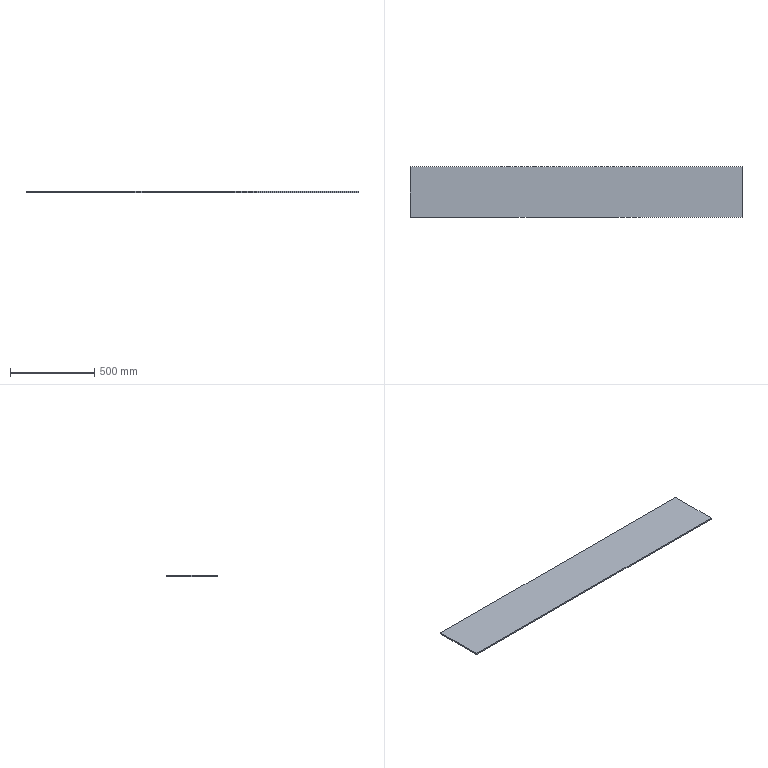Part | SolidWorks | features BaseBody 1, MoveFace 1 | 1 solid | 6 faces | box 1968 x 300 x 8 mm | volume 4723200 mm3 | plane 6
STEP:
#1=CARTESIAN_POINT('',(0.,0.,0.));
#2=VERTEX_POINT('',#1);
#3=CARTESIAN_POINT('',(1968.,0.,0.));
#4=VERTEX_POINT('',#3);
#5=CARTESIAN_POINT('',(0.,0.,0.));
#6=DIRECTION('',(1.,0.,0.));
#7=VECTOR('',#6,1000.);
#8=LINE('',#5,#7);
#9=EDGE_CURVE('',#2,#4,#8,.T.);
#10=ORIENTED_EDGE('',*,*,#9,.F.);
#11=CARTESIAN_POINT('',(0.,300.,0.));
#12=VERTEX_POINT('',#11);
#13=CARTESIAN_POINT('',(0.,300.,0.));
#14=DIRECTION('',(0.,-1.,0.));
#15=VECTOR('',#14,1000.);
#16=LINE('',#13,#15);
#17=EDGE_CURVE('',#12,#2,#16,.T.);
#18=ORIENTED_EDGE('',*,*,#17,.F.);
#19=CARTESIAN_POINT('',(1968.,300.,0.));
#20=VERTEX_POINT('',#19);
#21=CARTESIAN_POINT('',(1970.,300.,0.));
#22=DIRECTION('',(-1.,0.,0.));
#23=VECTOR('',#22,1000.);
#24=LINE('',#21,#23);
#25=EDGE_CURVE('',#20,#12,#24,.T.);
#26=ORIENTED_EDGE('',*,*,#25,.F.);
#27=CARTESIAN_POINT('',(1968.,0.,0.));
#28=DIRECTION('',(0.,1.,0.));
#29=VECTOR('',#28,1000.);
#30=LINE('',#27,#29);
#31=EDGE_CURVE('',#4,#20,#30,.T.);
#32=ORIENTED_EDGE('',*,*,#31,.F.);
#33=EDGE_LOOP('',(#10,#18,#26,#32));
#34=FACE_OUTER_BOUND('',#33,.T.);
#35=CARTESIAN_POINT('',(985.,150.,0.));
#36=DIRECTION('',(0.,0.,1.));
#37=DIRECTION('',(1.,0.,0.));
#38=AXIS2_PLACEMENT_3D('',#35,#36,#37);
#39=PLANE('',#38);
#40=ADVANCED_FACE('',(#34),#39,.F.);
#41=CARTESIAN_POINT('',(0.,0.,8.));
#42=VERTEX_POINT('',#41);
#43=CARTESIAN_POINT('',(1968.,0.,8.));
#44=VERTEX_POINT('',#43);
#45=CARTESIAN_POINT('',(0.,0.,8.));
#46=DIRECTION('',(1.,0.,0.));
#47=VECTOR('',#46,1000.);
#48=LINE('',#45,#47);
#49=EDGE_CURVE('',#42,#44,#48,.T.);
#50=ORIENTED_EDGE('',*,*,#49,.T.);
#51=CARTESIAN_POINT('',(1968.,300.,8.));
#52=VERTEX_POINT('',#51);
#53=CARTESIAN_POINT('',(1968.,0.,8.));
#54=DIRECTION('',(0.,1.,0.));
#55=VECTOR('',#54,1000.);
#56=LINE('',#53,#55);
#57=EDGE_CURVE('',#44,#52,#56,.T.);
#58=ORIENTED_EDGE('',*,*,#57,.T.);
#59=CARTESIAN_POINT('',(0.,300.,8.));
#60=VERTEX_POINT('',#59);
#61=CARTESIAN_POINT('',(1970.,300.,8.));
#62=DIRECTION('',(-1.,0.,0.));
#63=VECTOR('',#62,1000.);
#64=LINE('',#61,#63);
#65=EDGE_CURVE('',#52,#60,#64,.T.);
#66=ORIENTED_EDGE('',*,*,#65,.T.);
#67=CARTESIAN_POINT('',(0.,300.,8.));
#68=DIRECTION('',(0.,-1.,0.));
#69=VECTOR('',#68,1000.);
#70=LINE('',#67,#69);
#71=EDGE_CURVE('',#60,#42,#70,.T.);
#72=ORIENTED_EDGE('',*,*,#71,.T.);
#73=EDGE_LOOP('',(#50,#58,#66,#72));
#74=FACE_OUTER_BOUND('',#73,.T.);
#75=CARTESIAN_POINT('',(985.,150.,8.));
#76=DIRECTION('',(0.,0.,1.));
#77=DIRECTION('',(1.,0.,0.));
#78=AXIS2_PLACEMENT_3D('',#75,#76,#77);
#79=PLANE('',#78);
#80=ADVANCED_FACE('',(#74),#79,.T.);
#81=ORIENTED_EDGE('',*,*,#9,.T.);
#82=CARTESIAN_POINT('',(1968.,0.,0.));
#83=DIRECTION('',(0.,0.,1.));
#84=VECTOR('',#83,1000.);
#85=LINE('',#82,#84);
#86=EDGE_CURVE('',#4,#44,#85,.T.);
#87=ORIENTED_EDGE('',*,*,#86,.T.);
#88=ORIENTED_EDGE('',*,*,#49,.F.);
#89=CARTESIAN_POINT('',(0.,0.,0.));
#90=DIRECTION('',(0.,0.,1.));
#91=VECTOR('',#90,1000.);
#92=LINE('',#89,#91);
#93=EDGE_CURVE('',#2,#42,#92,.T.);
#94=ORIENTED_EDGE('',*,*,#93,.F.);
#95=EDGE_LOOP('',(#81,#87,#88,#94));
#96=FACE_OUTER_BOUND('',#95,.T.);
#97=CARTESIAN_POINT('',(0.,0.,0.));
#98=DIRECTION('',(0.,-1.,0.));
#99=DIRECTION('',(0.,0.,-1.));
#100=AXIS2_PLACEMENT_3D('',#97,#98,#99);
#101=PLANE('',#100);
#102=ADVANCED_FACE('',(#96),#101,.T.);
#103=ORIENTED_EDGE('',*,*,#31,.T.);
#104=CARTESIAN_POINT('',(1968.,300.,0.));
#105=DIRECTION('',(0.,0.,1.));
#106=VECTOR('',#105,1000.);
#107=LINE('',#104,#106);
#108=EDGE_CURVE('',#20,#52,#107,.T.);
#109=ORIENTED_EDGE('',*,*,#108,.T.);
#110=ORIENTED_EDGE('',*,*,#57,.F.);
#111=ORIENTED_EDGE('',*,*,#86,.F.);
#112=EDGE_LOOP('',(#103,#109,#110,#111));
#113=FACE_OUTER_BOUND('',#112,.T.);
#114=CARTESIAN_POINT('',(1968.,0.,0.));
#115=DIRECTION('',(1.,0.,0.));
#116=DIRECTION('',(0.,1.,0.));
#117=AXIS2_PLACEMENT_3D('',#114,#115,#116);
#118=PLANE('',#117);
#119=ADVANCED_FACE('',(#113),#118,.T.);
#120=ORIENTED_EDGE('',*,*,#25,.T.);
#121=CARTESIAN_POINT('',(0.,300.,0.));
#122=DIRECTION('',(0.,0.,1.));
#123=VECTOR('',#122,1000.);
#124=LINE('',#121,#123);
#125=EDGE_CURVE('',#12,#60,#124,.T.);
#126=ORIENTED_EDGE('',*,*,#125,.T.);
#127=ORIENTED_EDGE('',*,*,#65,.F.);
#128=ORIENTED_EDGE('',*,*,#108,.F.);
#129=EDGE_LOOP('',(#120,#126,#127,#128));
#130=FACE_OUTER_BOUND('',#129,.T.);
#131=CARTESIAN_POINT('',(1970.,300.,0.));
#132=DIRECTION('',(0.,1.,0.));
#133=DIRECTION('',(1.,0.,0.));
#134=AXIS2_PLACEMENT_3D('',#131,#132,#133);
#135=PLANE('',#134);
#136=ADVANCED_FACE('',(#130),#135,.T.);
#137=ORIENTED_EDGE('',*,*,#17,.T.);
#138=ORIENTED_EDGE('',*,*,#93,.T.);
#139=ORIENTED_EDGE('',*,*,#71,.F.);
#140=ORIENTED_EDGE('',*,*,#125,.F.);
#141=EDGE_LOOP('',(#137,#138,#139,#140));
#142=FACE_OUTER_BOUND('',#141,.T.);
#143=CARTESIAN_POINT('',(0.,300.,0.));
#144=DIRECTION('',(-1.,0.,0.));
#145=DIRECTION('',(0.,1.,0.));
#146=AXIS2_PLACEMENT_3D('',#143,#144,#145);
#147=PLANE('',#146);
#148=ADVANCED_FACE('',(#142),#147,.T.);
#149=CLOSED_SHELL('',(#40,#80,#102,#119,#136,#148));
#150=MANIFOLD_SOLID_BREP('',#149);
#151=CARTESIAN_POINT('',(0.,0.,0.));
#152=DIRECTION('',(0.,0.,1.));
#153=DIRECTION('',(1.,0.,0.));
#154=AXIS2_PLACEMENT_3D('',#151,#152,#153);
#155=(LENGTH_UNIT()NAMED_UNIT(*)SI_UNIT(.MILLI.,.METRE.));
#156=UNCERTAINTY_MEASURE_WITH_UNIT(LENGTH_MEASURE(0.00001),#155,'','');
#157=(NAMED_UNIT(*)PLANE_ANGLE_UNIT()SI_UNIT($,.RADIAN.));
#158=(NAMED_UNIT(*)SI_UNIT($,.STERADIAN.)SOLID_ANGLE_UNIT());
#159=(GEOMETRIC_REPRESENTATION_CONTEXT(3)GLOBAL_UNCERTAINTY_ASSIGNED_CONTEXT((#156))GLOBAL_UNIT_ASSIGNED_CONTEXT((#155,#157,#158))REPRESENTATION_CONTEXT('',''));
#160=ADVANCED_BREP_SHAPE_REPRESENTATION('',(#150,#154),#159);